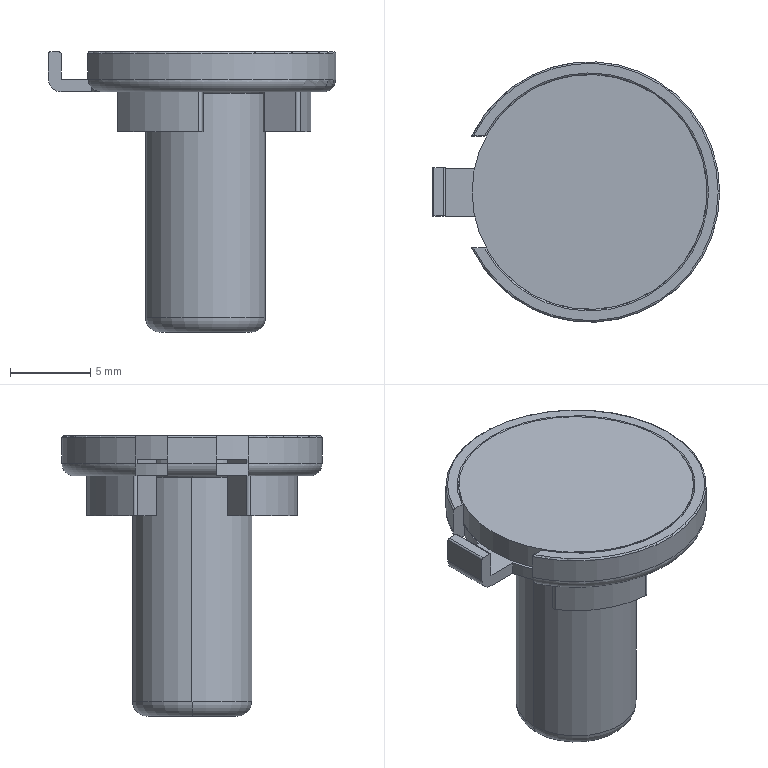NC program | NX | posted with a generic post | part box 17.958 x 16.273 x 17.5 mm
Lines 1 to 868 of 11029:
N10 G17 G21 G94 G90
(ZLEVEL_PROFILE_COPY_COPY_2_COPY , TOOL : D4)
N12 T04 M6
N14 G54
N16 G17 G0 G90 X-7.969 Y4.847 S6500 M3
N18 G43 Z30. H4
N20 Z1.
N22 G94 G1 X-7.675 Y5.315 Z0.971 F1800.
N24 X-7.407 Y5.691 Z0.947
N26 X-6.764 Y6.442 Z0.895
N28 X-6.434 Y6.764 Z0.871
N30 X-6.319 Y6.871 Z0.863
N32 X-5.712 Y7.384 Z0.821
N34 X-5.325 Y7.668 Z0.796
N36 X-4.924 Y7.931 Z0.771
N38 X-4.538 Y8.165 Z0.747
N40 X-3.72 Y8.566 Z0.699
N42 X-2.87 Y8.892 Z0.652
N44 X-2.436 Y9.016 Z0.628
N46 X-1.897 Y9.146 Z0.599
N48 X-1.864 Y9.153 Z0.597
N50 X-1.317 Y9.242 Z0.568
N52 X-0.844 Y9.297 Z0.543
N54 X-0.369 Y9.328 Z0.518
N56 X0.114 Y9.337 Z0.493
N58 X0.597 Y9.317 Z0.468
N60 X1.048 Y9.284 Z0.444
N62 X2.038 Y9.117 Z0.391
N64 X2.476 Y9.001 Z0.367
N66 X2.945 Y8.859 Z0.342
N68 X3.406 Y8.692 Z0.316
N70 X3.511 Y8.651 Z0.31
N72 X4.303 Y8.284 Z0.264
N74 X4.703 Y8.064 Z0.24
N76 X5.092 Y7.824 Z0.217
N78 X5.245 Y7.723 Z0.207
N80 X5.875 Y7.255 Z0.166
N82 X5.989 Y7.162 Z0.158
N84 X6.6 Y6.603 Z0.115
N86 X6.934 Y6.254 Z0.089
N88 X7.246 Y5.886 Z0.064
N90 X7.349 Y5.758 Z0.055
N92 X7.806 Y5.119 Z0.014
N94 X8.061 Y4.709 Z-0.011
N96 X8.294 Y4.286 Z-0.036
N98 X8.504 Y3.851 Z-0.062
N100 X8.692 Y3.406 Z-0.087
N102 X8.852 Y2.962 Z-0.112
N104 X8.991 Y2.511 Z-0.136
N106 X9.111 Y2.04 Z-0.162
N108 X9.204 Y1.562 Z-0.187
N110 X9.276 Y1.09 Z-0.212
N112 X9.315 Y0.614 Z-0.237
N114 X9.343 Y0.183 Z-0.26
N116 X9.303 Y-0.87 Z-0.315
N118 X9.243 Y-1.299 Z-0.338
N120 X9.175 Y-1.738 Z-0.361
N122 X9.076 Y-2.172 Z-0.385
N124 X9.043 Y-2.314
N126 G2 X8.415 Y-4.037 R9.789
N128 X7.753 Y-5.209 R13.022
N130 X6.449 Y-6.749 R10.24
N132 X5.519 Y-7.524 R8.875
N134 X3.916 Y-8.476 R9.811
N136 X2.739 Y-8.922 R11.518
N138 X0.843 Y-9.295 R9.159
N140 G1 X0.702 Y-9.309
N142 X-0.105 Y-9.332
N144 G2 X-1.071 Y-9.272 R13.937
N146 X-2.023 Y-9.112 R14.816
N148 X-2.945 Y-8.856 R14.576
N150 X-4.698 Y-8.065 R10.13
N152 G1 X-4.805 Y-8.004
N154 X-5.497 Y-7.543
N156 X-5.634 Y-7.443
N158 X-6.249 Y-6.932
N160 G2 X-7.832 Y-5.085 R10.033
N162 X-8.496 Y-3.862 R11.107
N164 G1 X-8.566 Y-3.711
N166 X-8.896 Y-2.842
N168 G2 X-9.27 Y-1.088 R9.715
N170 X-9.297 Y0.843 R10.387
N172 G1 X-9.283 Y0.983
N174 X-9.159 Y1.808
N176 X-9.128 Y1.963
N178 X-8.93 Y2.722
N180 G2 X-8.603 Y3.625 R13.087
N182 G1 X-8.529 Y3.792
N184 X-8.182 Y4.495
N186 X-8.103 Y4.634
N188 X-7.675 Y5.315
N190 G2 X-6.434 Y6.764 R10.615
N192 G1 X-6.319 Y6.871
N194 X-5.712 Y7.384
N196 G2 X-4.924 Y7.931 R18.201
N198 X-2.436 Y9.016 R10.177
N200 X-1.317 Y9.242 R15.371
N202 X-0.369 Y9.328 R18.827
N204 X0.597 Y9.317 R15.684
N206 X2.476 Y9.001 R10.229
N208 X3.406 Y8.692 R17.352
N210 G1 X3.511 Y8.651
N212 X4.303 Y8.284
N214 G2 X5.092 Y7.824 R19.463
N216 G1 X5.245 Y7.723
N218 X5.875 Y7.255
N220 X5.989 Y7.162
N222 X6.6 Y6.603
N224 G2 X7.246 Y5.886 R15.792
N226 G1 X7.349 Y5.758
N228 X7.806 Y5.119
N230 G2 X8.294 Y4.286 R18.161
N232 X8.692 Y3.406 R18.409
N234 X8.991 Y2.511 R19.157
N236 X9.204 Y1.562 R16.875
N238 X9.315 Y0.614 R13.353
N240 X9.243 Y-1.299 R9.36
N242 X9.076 Y-2.172 R12.725
N244 G1 X9.045 Y-2.31 Z-0.387
N246 X9.009 Y-2.446 Z-0.39
N248 X8.967 Y-2.581 Z-0.392
N250 X8.924 Y-2.715 Z-0.394
N252 X8.881 Y-2.85 Z-0.397
N254 X8.838 Y-2.984 Z-0.399
N256 X8.795 Y-3.119 Z-0.402
N258 X8.75 Y-3.253 Z-0.404
N260 X8.699 Y-3.385 Z-0.407
N262 X8.643 Y-3.514 Z-0.409
N264 X8.586 Y-3.644 Z-0.412
N266 X8.53 Y-3.773 Z-0.414
N268 X8.473 Y-3.903 Z-0.417
N270 X8.417 Y-4.032 Z-0.419
N272 X8.357 Y-4.16 Z-0.422
N274 X8.291 Y-4.285 Z-0.424
N276 X8.222 Y-4.409 Z-0.427
N278 X8.152 Y-4.531 Z-0.429
N280 X8.083 Y-4.654 Z-0.431
N282 X8.013 Y-4.777 Z-0.434
N284 X7.944 Y-4.9 Z-0.436
N286 X7.871 Y-5.021 Z-0.439
N288 X7.791 Y-5.138 Z-0.441
N290 X7.709 Y-5.252 Z-0.444
N292 X7.628 Y-5.368 Z-0.446
N294 X7.546 Y-5.482 Z-0.449
N296 X7.464 Y-5.598 Z-0.451
N298 X7.382 Y-5.713 Z-0.454
N300 X7.295 Y-5.824 Z-0.456
N302 X7.204 Y-5.932 Z-0.459
N304 X7.111 Y-6.038 Z-0.461
N306 X7.018 Y-6.144 Z-0.464
N308 X6.924 Y-6.25 Z-0.466
N310 X6.831 Y-6.356 Z-0.468
N312 X6.737 Y-6.462 Z-0.471
N314 X6.638 Y-6.563 Z-0.473
N316 X6.536 Y-6.66 Z-0.476
N318 X6.432 Y-6.756 Z-0.478
N320 X6.328 Y-6.851 Z-0.481
N322 X6.225 Y-6.947 Z-0.483
N324 X6.121 Y-7.043 Z-0.486
N326 X6.016 Y-7.138 Z-0.488
N328 X5.907 Y-7.228 Z-0.491
N330 X5.795 Y-7.313 Z-0.493
N332 X5.681 Y-7.397 Z-0.496
N334 X5.569 Y-7.482 Z-0.498
N336 X5.456 Y-7.567 Z-0.5
N338 X5.343 Y-7.652 Z-0.503
N340 X5.228 Y-7.734 Z-0.505
N342 X5.11 Y-7.811 Z-0.508
N344 X4.988 Y-7.884 Z-0.51
N346 X4.867 Y-7.957 Z-0.513
N348 X4.746 Y-8.029 Z-0.515
N350 X4.625 Y-8.102 Z-0.518
N352 X4.504 Y-8.174 Z-0.52
N354 X4.381 Y-8.244 Z-0.523
N356 X4.254 Y-8.307 Z-0.525
N358 X4.126 Y-8.367 Z-0.528
N360 X3.999 Y-8.426 Z-0.53
N362 X3.871 Y-8.486 Z-0.533
N364 X3.743 Y-8.546 Z-0.535
N366 X3.615 Y-8.606 Z-0.537
N368 X3.485 Y-8.66 Z-0.54
N370 X3.352 Y-8.709 Z-0.542
N372 X3.218 Y-8.755 Z-0.545
N374 X3.085 Y-8.802 Z-0.547
N376 X2.952 Y-8.848 Z-0.55
N378 X2.818 Y-8.895 Z-0.552
N380 X2.685 Y-8.94 Z-0.555
N382 X2.549 Y-8.981 Z-0.557
N384 X2.412 Y-9.014 Z-0.56
N386 X2.275 Y-9.047 Z-0.562
N388 X2.137 Y-9.079 Z-0.565
N390 X2. Y-9.111 Z-0.567
N392 X1.862 Y-9.144 Z-0.57
N394 X1.724 Y-9.174 Z-0.572
N396 X1.585 Y-9.2 Z-0.574
N398 X1.445 Y-9.218 Z-0.577
N400 X1.305 Y-9.236 Z-0.579
N402 X1.165 Y-9.254 Z-0.582
N404 X1.025 Y-9.272 Z-0.584
N406 X0.885 Y-9.29 Z-0.587
N408 X0.745 Y-9.305 Z-0.589
N410 X0.604 Y-9.314 Z-0.592
N412 X0.463 Y-9.318 Z-0.594
N414 X0.321 Y-9.322 Z-0.597
N416 X0.18 Y-9.325 Z-0.599
N418 X0.039 Y-9.329 Z-0.602
N420 X-0.102 Y-9.332 Z-0.604
N422 X-0.244 Z-0.607
N424 X-0.385 Y-9.325 Z-0.609
N426 X-0.526 Y-9.314 Z-0.611
N428 X-0.666 Y-9.303 Z-0.614
N430 X-0.807 Y-9.292 Z-0.616
N432 X-0.948 Y-9.281 Z-0.619
N434 X-1.089 Y-9.271 Z-0.621
N436 X-1.229 Y-9.254 Z-0.624
N438 X-1.369 Y-9.231 Z-0.626
N440 X-1.508 Y-9.206 Z-0.629
N442 X-1.647 Y-9.18 Z-0.631
N444 X-1.785 Y-9.155 Z-0.634
N446 X-1.924 Y-9.13 Z-0.636
N448 X-2.063 Y-9.104 Z-0.639
N450 X-2.201 Y-9.073 Z-0.641
N452 X-2.337 Y-9.034 Z-0.643
N454 X-2.473 Y-8.994 Z-0.646
N456 X-2.608 Y-8.955 Z-0.648
N458 X-2.744 Y-8.915 Z-0.651
N460 X-2.88 Y-8.876 Z-0.653
N462 X-3.015 Y-8.835 Z-0.656
N464 X-3.148 Y-8.788 Z-0.658
N466 X-3.279 Y-8.735 Z-0.661
N468 X-3.41 Y-8.682 Z-0.663
N470 X-3.541 Y-8.629 Z-0.666
N472 X-3.672 Y-8.576 Z-0.668
N474 X-3.803 Y-8.523 Z-0.671
N476 X-3.932 Y-8.467 Z-0.673
N478 X-4.06 Y-8.405 Z-0.676
N480 X-4.184 Y-8.339 Z-0.678
N482 X-4.309 Y-8.272 Z-0.68
N484 X-4.434 Y-8.206 Z-0.683
N486 X-4.558 Y-8.14 Z-0.685
N488 X-4.683 Y-8.073 Z-0.688
N490 X-4.806 Y-8.003 Z-0.69
N492 X-4.925 Y-7.928 Z-0.693
N494 X-5.042 Y-7.849 Z-0.695
N496 X-5.16 Y-7.77 Z-0.698
N498 X-5.277 Y-7.691 Z-0.7
N500 X-5.394 Y-7.612 Z-0.703
N502 X-5.511 Y-7.533 Z-0.705
N504 X-5.625 Y-7.45 Z-0.708
N506 X-5.735 Y-7.362 Z-0.71
N508 X-5.844 Y-7.271 Z-0.713
N510 X-5.952 Y-7.181 Z-0.715
N512 X-6.061 Y-7.09 Z-0.717
N514 X-6.169 Y-7. Z-0.72
N516 X-6.277 Y-6.909 Z-0.722
N518 X-6.382 Y-6.814 Z-0.725
N520 X-6.481 Y-6.713 Z-0.727
N522 X-6.58 Y-6.612 Z-0.73
N524 X-6.678 Y-6.511 Z-0.732
N526 X-6.777 Y-6.41 Z-0.735
N528 X-6.875 Y-6.308 Z-0.737
N530 X-6.974 Y-6.207 Z-0.74
N532 X-7.066 Y-6.1 Z-0.742
N534 X-7.154 Y-5.989 Z-0.745
N536 X-7.242 Y-5.879 Z-0.747
N538 X-7.329 Y-5.768 Z-0.75
N540 X-7.417 Y-5.657 Z-0.752
N542 X-7.505 Y-5.546 Z-0.754
N544 X-7.59 Y-5.434 Z-0.757
N546 X-7.671 Y-5.318 Z-0.759
N548 X-7.747 Y-5.199 Z-0.762
N550 X-7.823 Y-5.08 Z-0.764
N552 X-7.899 Y-4.961 Z-0.767
N554 X-7.979 Y-4.845 Z-0.769
N556 G2 X-8.496 Y-3.862 R11.006
N558 G1 X-8.566 Y-3.711
N560 X-8.896 Y-2.842
N562 G2 X-9.27 Y-1.088 R9.696
N564 X-9.297 Y0.843 R10.313
N566 G1 X-9.283 Y0.983
N568 X-9.159 Y1.808
N570 X-9.128 Y1.963
N572 X-8.93 Y2.722
N574 G2 X-8.603 Y3.625 R12.798
N576 G1 X-8.529 Y3.792
N578 X-8.182 Y4.495
N580 X-8.103 Y4.634
N582 X-7.675 Y5.315
N584 G2 X-6.434 Y6.764 R10.5
N586 G1 X-6.319 Y6.871
N588 X-5.712 Y7.384
N590 G2 X-4.924 Y7.931 R17.941
N592 X-2.977 Y8.848 R10.322
N594 G1 X-2.282 Y9.049
N596 X-2.265 Y9.057
N598 X-2.106 Y9.095
N600 X-1.317 Y9.242
N602 G2 X-0.369 Y9.328 R17.935
N604 X0.597 Y9.317 R15.041
N606 X2.476 Y9.001 R10.174
N608 X3.406 Y8.692 R16.786
N610 G1 X3.511 Y8.651
N612 X4.303 Y8.284
N614 G2 X5.092 Y7.824 R20.101
N616 G1 X5.245 Y7.723
N618 X5.875 Y7.255
N620 X5.989 Y7.162
N622 X6.6 Y6.603
N624 G2 X7.246 Y5.886 R15.35
N626 G1 X7.349 Y5.758
N628 X7.806 Y5.119
N630 G2 X8.294 Y4.286 R13.93
N632 X8.692 Y3.406 R18.133
N634 X8.991 Y2.511 R18.296
N636 X9.204 Y1.562 R14.845
N638 X9.315 Y0.614 R13.007
N640 X9.243 Y-1.299 R9.344
N642 X9.077 Y-2.172 R10.569
N644 G1 X9.045 Y-2.31 Z-0.772
N646 X9.009 Y-2.446 Z-0.774
N648 X8.967 Y-2.581 Z-0.777
N650 X8.924 Y-2.716 Z-0.779
N652 X8.881 Y-2.85 Z-0.782
N654 X8.838 Y-2.985 Z-0.784
N656 X8.795 Y-3.119 Z-0.786
N658 X8.75 Y-3.253 Z-0.789
N660 X8.7 Y-3.385 Z-0.791
N662 X8.643 Y-3.515 Z-0.794
N664 X8.586 Y-3.644 Z-0.796
N666 X8.53 Y-3.773 Z-0.799
N668 X8.473 Y-3.903 Z-0.801
N670 X8.417 Y-4.032 Z-0.804
N672 X8.357 Y-4.16 Z-0.806
N674 X8.292 Y-4.285 Z-0.809
N676 X8.222 Y-4.408 Z-0.811
N678 X8.153 Y-4.531 Z-0.814
N680 X8.083 Y-4.654 Z-0.816
N682 X8.013 Y-4.777 Z-0.819
N684 X7.944 Y-4.9 Z-0.821
N686 X7.871 Y-5.021 Z-0.823
N688 X7.791 Y-5.137 Z-0.826
N690 X7.71 Y-5.253 Z-0.828
N692 X7.627 Y-5.368 Z-0.831
N694 X7.546 Y-5.483 Z-0.833
N696 X7.464 Y-5.598 Z-0.836
N698 X7.382 Y-5.713 Z-0.838
N700 X7.295 Y-5.825 Z-0.841
N702 X7.204 Y-5.932 Z-0.843
N704 X7.11 Y-6.038 Z-0.846
N706 X7.017 Y-6.144 Z-0.848
N708 X6.924 Y-6.25 Z-0.851
N710 X6.831 Y-6.356 Z-0.853
N712 X6.737 Y-6.462 Z-0.856
N714 X6.639 Y-6.564 Z-0.858
N716 X6.535 Y-6.66 Z-0.86
N718 X6.432 Y-6.756 Z-0.863
N720 X6.328 Y-6.852 Z-0.865
N722 X6.225 Y-6.948 Z-0.868
N724 X6.121 Y-7.044 Z-0.87
N726 X6.016 Y-7.138 Z-0.873
N728 X5.907 Y-7.228 Z-0.875
N730 X5.794 Y-7.313 Z-0.878
N732 X5.681 Y-7.398 Z-0.88
N734 X5.568 Y-7.483 Z-0.883
N736 X5.455 Y-7.567 Z-0.885
N738 X5.342 Y-7.652 Z-0.888
N740 X5.227 Y-7.734 Z-0.89
N742 X5.109 Y-7.812 Z-0.893
N744 X4.988 Y-7.884 Z-0.895
N746 X4.867 Y-7.957 Z-0.897
N748 X4.746 Y-8.029 Z-0.9
N750 X4.625 Y-8.102 Z-0.902
N752 X4.503 Y-8.175 Z-0.905
N754 X4.38 Y-8.244 Z-0.907
N756 X4.254 Y-8.307 Z-0.91
N758 X4.126 Y-8.367 Z-0.912
N760 X3.998 Y-8.427 Z-0.915
N762 X3.87 Y-8.487 Z-0.917
N764 X3.742 Y-8.547 Z-0.92
N766 X3.614 Y-8.607 Z-0.922
N768 X3.484 Y-8.661 Z-0.925
N770 X3.351 Y-8.709 Z-0.927
N772 X3.218 Y-8.756 Z-0.929
N774 X3.084 Y-8.803 Z-0.932
N776 X2.951 Y-8.849 Z-0.934
N778 X2.817 Y-8.895 Z-0.937
N780 X2.684 Y-8.941 Z-0.939
N782 X2.548 Y-8.981 Z-0.942
N784 X2.411 Y-9.014 Z-0.944
N786 X2.273 Y-9.047 Z-0.947
N788 X2.136 Y-9.079 Z-0.949
N790 X1.999 Y-9.112 Z-0.952
N792 X1.861 Y-9.144 Z-0.954
N794 X1.723 Y-9.174 Z-0.957
N796 X1.584 Y-9.199 Z-0.959
N798 X1.444 Y-9.218 Z-0.962
N800 X1.304 Y-9.236 Z-0.964
N802 X1.164 Y-9.254 Z-0.966
N804 X1.024 Y-9.272 Z-0.969
N806 X0.884 Y-9.291 Z-0.971
N808 X0.743 Y-9.305 Z-0.974
N810 X0.602 Y-9.315 Z-0.976
N812 X0.461 Y-9.318 Z-0.979
N814 X0.32 Y-9.322 Z-0.981
N816 X0.179 Y-9.325 Z-0.984
N818 X0.038 Y-9.329 Z-0.986
N820 X-0.104 Y-9.333 Z-0.989
N822 X-0.245 Y-9.332 Z-0.991
N824 X-0.386 Y-9.325 Z-0.994
N826 X-0.527 Y-9.314 Z-0.996
N828 X-0.668 Y-9.303 Z-0.999
N830 X-0.808 Y-9.293 Z-1.001
N832 X-0.949 Y-9.282 Z-1.003
N834 X-1.09 Y-9.271 Z-1.006
N836 X-1.23 Y-9.254 Z-1.008
N838 X-1.37 Y-9.231 Z-1.011
N840 X-1.509 Y-9.206 Z-1.013
N842 X-1.648 Y-9.18 Z-1.016
N844 X-1.787 Y-9.155 Z-1.018
N846 X-1.926 Y-9.13 Z-1.021
N848 X-2.065 Y-9.104 Z-1.023
N850 X-2.202 Y-9.071 Z-1.026
N852 X-2.338 Y-9.034 Z-1.028
N854 X-2.474 Y-8.994 Z-1.031
N856 X-2.609 Y-8.955 Z-1.033
N858 X-2.745 Y-8.915 Z-1.036
N860 X-2.881 Y-8.875 Z-1.038
N862 X-3.016 Y-8.834 Z-1.04
N864 X-3.149 Y-8.788 Z-1.043
N866 X-3.28 Y-8.735 Z-1.045
N868 X-3.411 Y-8.682 Z-1.048
N870 X-3.542 Y-8.628 Z-1.05
N872 X-3.673 Y-8.575 Z-1.053
N874 X-3.803 Y-8.522 Z-1.055
N876 X-3.933 Y-8.466 Z-1.058
N878 X-4.061 Y-8.405 Z-1.06
N880 X-4.185 Y-8.338 Z-1.063
N882 X-4.31 Y-8.272 Z-1.065
N884 X-4.435 Y-8.206 Z-1.068
N886 X-4.559 Y-8.139 Z-1.07
N888 X-4.684 Y-8.073 Z-1.072
N890 X-4.807 Y-8.003 Z-1.075
N892 X-4.926 Y-7.927 Z-1.077
N894 X-5.043 Y-7.849 Z-1.08
N896 X-5.16 Y-7.77 Z-1.082
N898 X-5.278 Y-7.691 Z-1.085
N900 X-5.395 Y-7.612 Z-1.087
N902 X-5.512 Y-7.533 Z-1.09
N904 X-5.626 Y-7.449 Z-1.092
N906 X-5.736 Y-7.361 Z-1.095
N908 X-5.845 Y-7.271 Z-1.097
N910 X-5.953 Y-7.18 Z-1.1
N912 X-6.062 Y-7.09 Z-1.102
N914 X-6.17 Y-6.999 Z-1.105
N916 X-6.278 Y-6.908 Z-1.107
N918 X-6.383 Y-6.813 Z-1.109
N920 X-6.482 Y-6.713 Z-1.112
N922 X-6.581 Y-6.611 Z-1.114
N924 X-6.679 Y-6.51 Z-1.117
N926 X-6.778 Y-6.409 Z-1.119
N928 X-6.876 Y-6.308 Z-1.122
N930 X-6.974 Y-6.206 Z-1.124
N932 X-7.067 Y-6.1 Z-1.127
N934 X-7.155 Y-5.989 Z-1.129
N936 X-7.243 Y-5.878 Z-1.132
N938 X-7.33 Y-5.767 Z-1.134
N940 X-7.418 Y-5.657 Z-1.137
N942 X-7.505 Y-5.546 Z-1.139
N944 X-7.591 Y-5.433 Z-1.142
N946 X-7.672 Y-5.318 Z-1.144
N948 X-7.748 Y-5.198 Z-1.146
N950 X-7.823 Y-5.079 Z-1.149
N952 X-7.899 Y-4.96 Z-1.151
N954 X-7.981 Y-4.845 Z-1.154
N956 G2 X-8.496 Y-3.862 R9.442
N958 G1 X-8.566 Y-3.711
N960 X-8.896 Y-2.842
N962 G2 X-9.319 Y0.615 R9.669
N964 X-9.159 Y1.808 R13.506
N966 G1 X-9.128 Y1.963
N968 X-8.93 Y2.722
N970 G2 X-8.603 Y3.625 R12.521
N972 G1 X-8.529 Y3.792
N974 X-8.182 Y4.495
N976 X-8.103 Y4.634
N978 X-7.675 Y5.315
N980 G2 X-6.434 Y6.764 R10.422
N982 G1 X-6.319 Y6.871
N984 X-5.712 Y7.384
N986 G2 X-4.924 Y7.931 R17.936
N988 X-2.512 Y8.997 R10.268
N990 X-1.317 Y9.242 R14.545
N992 X-0.369 Y9.328 R17.03
N994 X0.597 Y9.317 R16.938
N996 X2.476 Y9.001 R10.581
N998 X3.406 Y8.692 R16.256
N1000 G1 X3.511 Y8.651
N1002 X4.303 Y8.284
N1004 G2 X5.092 Y7.824 R19.214
N1006 G1 X5.245 Y7.723
N1008 X5.875 Y7.255
N1010 X5.989 Y7.162
N1012 X6.6 Y6.603
N1014 G2 X7.246 Y5.886 R14.932
N1016 G1 X7.349 Y5.758
N1018 X7.806 Y5.119
N1020 G2 X8.294 Y4.286 R13.639
N1022 X8.692 Y3.406 R17.441
N1024 X8.991 Y2.511 R16.046
N1026 G1 X9.026 Y2.387
N1028 X9.204 Y1.562
N1030 G2 X9.315 Y0.614 R16.29
N1032 X9.079 Y-2.172 R9.512
N1034 G1 X9.045 Y-2.31 Z-1.156
N1036 X9.009 Y-2.446 Z-1.159
N1038 X8.967 Y-2.581 Z-1.161
N1040 X8.924 Y-2.716 Z-1.164
N1042 X8.881 Y-2.85 Z-1.166
N1044 X8.838 Y-2.984 Z-1.169
N1046 X8.795 Y-3.119 Z-1.171
N1048 X8.751 Y-3.253 Z-1.174
N1050 X8.699 Y-3.385 Z-1.176
N1052 X8.643 Y-3.515 Z-1.179
N1054 X8.587 Y-3.644 Z-1.181
N1056 X8.53 Y-3.773 Z-1.183
N1058 X8.474 Y-3.903 Z-1.186
N1060 X8.417 Y-4.032 Z-1.188
N1062 X8.357 Y-4.16 Z-1.191
N1064 X8.292 Y-4.285 Z-1.193
N1066 X8.222 Y-4.408 Z-1.196
N1068 X8.153 Y-4.531 Z-1.198
N1070 X8.083 Y-4.654 Z-1.201
N1072 X8.014 Y-4.777 Z-1.203
N1074 X7.944 Y-4.9 Z-1.206
N1076 X7.871 Y-5.021 Z-1.208
N1078 X7.791 Y-5.137 Z-1.211
N1080 X7.709 Y-5.253 Z-1.213
N1082 X7.628 Y-5.368 Z-1.215
N1084 X7.546 Y-5.483 Z-1.218
N1086 X7.464 Y-5.598 Z-1.22
N1088 X7.382 Y-5.713 Z-1.223
N1090 X7.295 Y-5.825 Z-1.225
N1092 X7.204 Y-5.932 Z-1.228
N1094 X7.111 Y-6.038 Z-1.23
N1096 X7.017 Y-6.144 Z-1.233
N1098 X6.924 Y-6.25 Z-1.235
N1100 X6.831 Y-6.356 Z-1.238
N1102 X6.737 Y-6.462 Z-1.24
N1104 X6.639 Y-6.564 Z-1.243
N1106 X6.536 Y-6.66 Z-1.245
N1108 X6.432 Y-6.756 Z-1.248
N1110 X6.328 Y-6.852 Z-1.25
N1112 X6.225 Y-6.948 Z-1.252
N1114 X6.121 Y-7.044 Z-1.255
N1116 X6.016 Y-7.139 Z-1.257
N1118 X5.907 Y-7.228 Z-1.26
N1120 X5.794 Y-7.313 Z-1.262
N1122 X5.681 Y-7.398 Z-1.265
N1124 X5.568 Y-7.483 Z-1.267
N1126 X5.455 Y-7.568 Z-1.27
N1128 X5.342 Y-7.652 Z-1.272
N1130 X5.227 Y-7.734 Z-1.275
N1132 X5.109 Y-7.812 Z-1.277
N1134 X4.988 Y-7.884 Z-1.28
N1136 X4.867 Y-7.957 Z-1.282
N1138 X4.746 Y-8.03 Z-1.285
N1140 X4.625 Y-8.102 Z-1.287
N1142 X4.504 Y-8.175 Z-1.289
N1144 X4.38 Y-8.244 Z-1.292
N1146 X4.254 Y-8.307 Z-1.294
N1148 X4.126 Y-8.367 Z-1.297
N1150 X3.998 Y-8.427 Z-1.299
N1152 X3.87 Y-8.487 Z-1.302
N1154 X3.742 Y-8.547 Z-1.304
N1156 X3.614 Y-8.606 Z-1.307
N1158 X3.484 Y-8.661 Z-1.309
N1160 X3.352 Y-8.709 Z-1.312
N1162 X3.218 Y-8.756 Z-1.314
N1164 X3.085 Y-8.802 Z-1.317
N1166 X2.952 Y-8.849 Z-1.319
N1168 X2.818 Y-8.895 Z-1.322
N1170 X2.685 Y-8.94 Z-1.324
N1172 X2.549 Y-8.981 Z-1.326
N1174 X2.412 Y-9.014 Z-1.329
N1176 X2.274 Y-9.046 Z-1.331
N1178 X2.137 Y-9.079 Z-1.334
N1180 X2. Y-9.111 Z-1.336
N1182 X1.862 Y-9.144 Z-1.339
N1184 X1.724 Y-9.174 Z-1.341
N1186 X1.585 Y-9.2 Z-1.344
N1188 X1.445 Y-9.218 Z-1.346
N1190 X1.305 Y-9.236 Z-1.349
N1192 X1.165 Y-9.254 Z-1.351
N1194 X1.025 Y-9.272 Z-1.354
N1196 X0.885 Y-9.291 Z-1.356
N1198 X0.744 Y-9.306 Z-1.358
N1200 X0.603 Y-9.315 Z-1.361
N1202 X0.462 Y-9.319 Z-1.363
N1204 X0.321 Y-9.322 Z-1.366
N1206 X0.18 Y-9.326 Z-1.368
N1208 X0.039 Y-9.329 Z-1.371
N1210 X-0.102 Y-9.333 Z-1.373
N1212 X-0.244 Y-9.332 Z-1.376
N1214 X-0.385 Y-9.325 Z-1.378
N1216 X-0.526 Y-9.315 Z-1.381
N1218 X-0.666 Y-9.303 Z-1.383
N1220 X-0.807 Y-9.292 Z-1.386
N1222 X-0.948 Y-9.282 Z-1.388
N1224 X-1.089 Y-9.271 Z-1.391
N1226 X-1.229 Y-9.254 Z-1.393
N1228 X-1.369 Y-9.231 Z-1.395
N1230 X-1.508 Y-9.206 Z-1.398
N1232 X-1.647 Y-9.181 Z-1.4
N1234 X-1.786 Y-9.155 Z-1.403
N1236 X-1.924 Y-9.13 Z-1.405
N1238 X-2.064 Y-9.105 Z-1.408
N1240 X-2.201 Y-9.072 Z-1.41
N1242 X-2.337 Y-9.034 Z-1.413
N1244 X-2.473 Y-8.995 Z-1.415
N1246 X-2.608 Y-8.955 Z-1.418
N1248 X-2.744 Y-8.916 Z-1.42
N1250 X-2.88 Y-8.876 Z-1.423
N1252 X-3.015 Y-8.835 Z-1.425
N1254 X-3.148 Y-8.788 Z-1.428
N1256 X-3.279 Y-8.736 Z-1.43
N1258 X-3.41 Y-8.682 Z-1.432
N1260 X-3.541 Y-8.629 Z-1.435
N1262 X-3.672 Y-8.576 Z-1.437
N1264 X-3.802 Y-8.523 Z-1.44
N1266 X-3.932 Y-8.467 Z-1.442
N1268 X-4.06 Y-8.405 Z-1.445
N1270 X-4.184 Y-8.339 Z-1.447
N1272 X-4.309 Y-8.272 Z-1.45
N1274 X-4.434 Y-8.206 Z-1.452
N1276 X-4.558 Y-8.14 Z-1.455
N1278 X-4.683 Y-8.073 Z-1.457
N1280 X-4.806 Y-8.003 Z-1.46
N1282 X-4.925 Y-7.928 Z-1.462
N1284 X-5.042 Y-7.849 Z-1.464
N1286 X-5.16 Y-7.77 Z-1.467
N1288 X-5.277 Y-7.692 Z-1.469
N1290 X-5.394 Y-7.612 Z-1.472
N1292 X-5.511 Y-7.534 Z-1.474
N1294 X-5.625 Y-7.45 Z-1.477
N1296 X-5.735 Y-7.362 Z-1.479
N1298 X-5.844 Y-7.272 Z-1.482
N1300 X-5.952 Y-7.181 Z-1.484
N1302 X-6.061 Y-7.091 Z-1.487
N1304 X-6.169 Y-7. Z-1.489
N1306 X-6.277 Y-6.909 Z-1.492
N1308 X-6.382 Y-6.814 Z-1.494
N1310 X-6.481 Y-6.714 Z-1.497
N1312 X-6.58 Y-6.612 Z-1.499
N1314 X-6.678 Y-6.511 Z-1.501
N1316 X-6.777 Y-6.41 Z-1.504
N1318 X-6.876 Y-6.309 Z-1.506
N1320 X-6.973 Y-6.207 Z-1.509
N1322 X-7.066 Y-6.101 Z-1.511
N1324 X-7.154 Y-5.99 Z-1.514
N1326 X-7.242 Y-5.879 Z-1.516
N1328 X-7.33 Y-5.768 Z-1.519
N1330 X-7.417 Y-5.658 Z-1.521
N1332 X-7.505 Y-5.547 Z-1.524
N1334 X-7.59 Y-5.434 Z-1.526
N1336 X-7.671 Y-5.319 Z-1.529
N1338 X-7.747 Y-5.199 Z-1.531
N1340 X-7.823 Y-5.08 Z-1.534
N1342 X-7.899 Y-4.961 Z-1.536
N1344 X-7.979 Y-4.845 Z-1.538
N1346 G2 X-8.496 Y-3.862 R10.917
N1348 G1 X-8.566 Y-3.711
N1350 X-8.896 Y-2.842
N1352 G2 X-9.27 Y-1.088 R9.877
N1354 X-9.297 Y0.843 R10.167
N1356 G1 X-9.283 Y0.983
N1358 X-9.159 Y1.808
N1360 X-9.128 Y1.963
N1362 X-8.93 Y2.722
N1364 G2 X-8.603 Y3.625 R15.769
N1366 G1 X-8.529 Y3.792
N1368 X-8.182 Y4.495
N1370 X-8.103 Y4.634
N1372 X-7.675 Y5.315
N1374 G2 X-6.434 Y6.764 R10.337
N1376 G1 X-6.319 Y6.871
N1378 X-5.712 Y7.384
N1380 G2 X-4.924 Y7.931 R17.284
N1382 X-2.511 Y8.997 R10.25
N1384 X-1.317 Y9.242 R14.291
N1386 X-0.369 Y9.328 R16.212
N1388 X0.597 Y9.317 R16.134
N1390 X2.476 Y9.001 R10.558
N1392 X3.406 Y8.692 R15.758
N1394 G1 X3.511 Y8.651
N1396 X4.303 Y8.284
N1398 G2 X5.092 Y7.824 R18.402
N1400 G1 X5.245 Y7.723
N1402 X5.875 Y7.255
N1404 X5.989 Y7.162
N1406 X6.6 Y6.603
N1408 G2 X7.246 Y5.886 R15.797
N1410 G1 X7.349 Y5.758
N1412 X7.806 Y5.119
N1414 G2 X8.294 Y4.286 R13.359
N1416 X8.692 Y3.406 R16.8
N1418 X8.991 Y2.511 R15.491
N1420 G1 X9.026 Y2.387
N1422 X9.204 Y1.562
N1424 G2 X9.315 Y0.614 R15.667
N1426 X9.077 Y-2.172 R9.413
N1428 G1 X9.045 Y-2.309 Z-1.541
N1430 X9.009 Y-2.446 Z-1.543
N1432 X8.967 Y-2.581 Z-1.546
N1434 X8.924 Y-2.716 Z-1.548
N1436 X8.881 Y-2.85 Z-1.551
N1438 X8.838 Y-2.985 Z-1.553
N1440 X8.795 Y-3.119 Z-1.556
N1442 X8.75 Y-3.253 Z-1.558
N1444 X8.699 Y-3.385 Z-1.561
N1446 X8.643 Y-3.515 Z-1.563
N1448 X8.586 Y-3.644 Z-1.566
N1450 X8.53 Y-3.773 Z-1.568
N1452 X8.474 Y-3.903 Z-1.571
N1454 X8.417 Y-4.032 Z-1.573
N1456 X8.357 Y-4.16 Z-1.575
N1458 X8.292 Y-4.286 Z-1.578
N1460 X8.222 Y-4.408 Z-1.58
N1462 X8.153 Y-4.531 Z-1.583
N1464 X8.083 Y-4.654 Z-1.585
N1466 X8.014 Y-4.777 Z-1.588
N1468 X7.944 Y-4.9 Z-1.59
N1470 X7.871 Y-5.021 Z-1.593
N1472 X7.791 Y-5.138 Z-1.595
N1474 X7.71 Y-5.253 Z-1.598
N1476 X7.628 Y-5.368 Z-1.6
N1478 X7.546 Y-5.483 Z-1.603
N1480 X7.464 Y-5.598 Z-1.605
N1482 X7.382 Y-5.713 Z-1.607
N1484 X7.295 Y-5.825 Z-1.61
N1486 X7.204 Y-5.932 Z-1.612
N1488 X7.111 Y-6.038 Z-1.615
N1490 X7.018 Y-6.145 Z-1.617
N1492 X6.924 Y-6.25 Z-1.62
N1494 X6.831 Y-6.357 Z-1.622
N1496 X6.737 Y-6.462 Z-1.625
N1498 X6.638 Y-6.563 Z-1.627
N1500 X6.536 Y-6.66 Z-1.63
N1502 X6.432 Y-6.756 Z-1.632
N1504 X6.328 Y-6.852 Z-1.635
N1506 X6.225 Y-6.948 Z-1.637
N1508 X6.121 Y-7.044 Z-1.64
N1510 X6.016 Y-7.138 Z-1.642
N1512 X5.907 Y-7.228 Z-1.644
N1514 X5.794 Y-7.313 Z-1.647
N1516 X5.681 Y-7.398 Z-1.649
N1518 X5.568 Y-7.483 Z-1.652
N1520 X5.455 Y-7.568 Z-1.654
N1522 X5.342 Y-7.652 Z-1.657
N1524 X5.228 Y-7.734 Z-1.659
N1526 X5.109 Y-7.812 Z-1.662
N1528 X4.988 Y-7.884 Z-1.664
N1530 X4.867 Y-7.957 Z-1.667
N1532 X4.746 Y-8.03 Z-1.669
N1534 X4.625 Y-8.102 Z-1.672
N1536 X4.504 Y-8.175 Z-1.674
N1538 X4.381 Y-8.244 Z-1.677
N1540 X4.254 Y-8.307 Z-1.679
N1542 X4.126 Y-8.367 Z-1.681
N1544 X3.998 Y-8.427 Z-1.684
N1546 X3.871 Y-8.487 Z-1.686
N1548 X3.743 Y-8.547 Z-1.689
N1550 X3.615 Y-8.606 Z-1.691
N1552 X3.484 Y-8.661 Z-1.694
N1554 X3.352 Y-8.709 Z-1.696
N1556 X3.218 Y-8.756 Z-1.699
N1558 X3.085 Y-8.803 Z-1.701
N1560 X2.951 Y-8.848 Z-1.704
N1562 X2.818 Y-8.895 Z-1.706
N1564 X2.684 Y-8.941 Z-1.709
N1566 X2.549 Y-8.981 Z-1.711
N1568 X2.412 Y-9.014 Z-1.714
N1570 X2.274 Y-9.047 Z-1.716
N1572 X2.137 Y-9.079 Z-1.718
N1574 X1.999 Y-9.112 Z-1.721
N1576 X1.862 Y-9.144 Z-1.723
N1578 X1.724 Y-9.175 Z-1.726
N1580 X1.585 Y-9.199 Z-1.728
N1582 X1.445 Y-9.218 Z-1.731
N1584 X1.305 Y-9.236 Z-1.733
N1586 X1.165 Y-9.254 Z-1.736
N1588 X1.025 Y-9.273 Z-1.738
N1590 X0.885 Y-9.291 Z-1.741
N1592 X0.744 Y-9.306 Z-1.743
N1594 X0.603 Y-9.315 Z-1.746
N1596 X0.462 Y-9.318 Z-1.748
N1598 X0.321 Y-9.322 Z-1.75
N1600 X0.18 Y-9.326 Z-1.753
N1602 X0.039 Y-9.33 Z-1.755
N1604 X-0.103 Y-9.333 Z-1.758
N1606 X-0.244 Y-9.332 Z-1.76
N1608 X-0.385 Y-9.326 Z-1.763
N1610 X-0.526 Y-9.314 Z-1.765
N1612 X-0.667 Y-9.304 Z-1.768
N1614 X-0.807 Y-9.293 Z-1.77
N1616 X-0.948 Y-9.281 Z-1.773
N1618 X-1.089 Y-9.271 Z-1.775
N1620 X-1.229 Y-9.254 Z-1.778
N1622 X-1.369 Y-9.231 Z-1.78
N1624 X-1.508 Y-9.206 Z-1.783
N1626 X-1.646 Y-9.181 Z-1.785
N1628 X-1.785 Y-9.156 Z-1.787
N1630 X-1.924 Y-9.13 Z-1.79
N1632 X-2.063 Y-9.104 Z-1.792
N1634 X-2.201 Y-9.072 Z-1.795
N1636 X-2.337 Y-9.034 Z-1.797
N1638 X-2.472 Y-8.995 Z-1.8
N1640 X-2.608 Y-8.955 Z-1.802
N1642 X-2.743 Y-8.916 Z-1.805
N1644 X-2.879 Y-8.876 Z-1.807
N1646 X-3.014 Y-8.836 Z-1.81
N1648 X-3.148 Y-8.788 Z-1.812
N1650 X-3.279 Y-8.736 Z-1.815
N1652 X-3.41 Y-8.682 Z-1.817
N1654 X-3.54 Y-8.629 Z-1.82
N1656 X-3.671 Y-8.576 Z-1.822
N1658 X-3.802 Y-8.523 Z-1.824
N1660 X-3.932 Y-8.467 Z-1.827
N1662 X-4.059 Y-8.406 Z-1.829
N1664 X-4.184 Y-8.339 Z-1.832
N1666 X-4.309 Y-8.273 Z-1.834
N1668 X-4.433 Y-8.206 Z-1.837
N1670 X-4.558 Y-8.14 Z-1.839
N1672 X-4.683 Y-8.074 Z-1.842
N1674 X-4.805 Y-8.004 Z-1.844
N1676 X-4.925 Y-7.929 Z-1.847
N1678 X-5.042 Y-7.85 Z-1.849
N1680 X-5.159 Y-7.771 Z-1.852
N1682 X-5.276 Y-7.692 Z-1.854
N1684 X-5.393 Y-7.613 Z-1.857
N1686 X-5.511 Y-7.535 Z-1.859
N1688 X-5.624 Y-7.451 Z-1.861
N1690 X-5.735 Y-7.363 Z-1.864
N1692 X-5.843 Y-7.272 Z-1.866
N1694 X-5.951 Y-7.182 Z-1.869
N1696 X-6.06 Y-7.092 Z-1.871
N1698 X-6.168 Y-7.001 Z-1.874
N1700 X-6.276 Y-6.91 Z-1.876
N1702 X-6.38 Y-6.815 Z-1.879
N1704 X-6.48 Y-6.715 Z-1.881
N1706 X-6.579 Y-6.614 Z-1.884
N1708 X-6.677 Y-6.513 Z-1.886
N1710 X-6.776 Y-6.411 Z-1.889
N1712 X-6.875 Y-6.31 Z-1.891
N1714 X-6.972 Y-6.208 Z-1.893
N1716 X-7.065 Y-6.102 Z-1.896
N1718 X-7.153 Y-5.991 Z-1.898
N1720 X-7.241 Y-5.88 Z-1.901
N1722 X-7.329 Y-5.77 Z-1.903
N1724 X-7.416 Y-5.659 Z-1.906
N1726 X-7.504 Y-5.548 Z-1.908
N1728 X-7.589 Y-5.436 Z-1.911
N1730 X-7.67 Y-5.32 Z-1.913
N1732 X-7.746 Y-5.201 Z-1.916
N1734 X-7.822 Y-5.082 Z-1.918